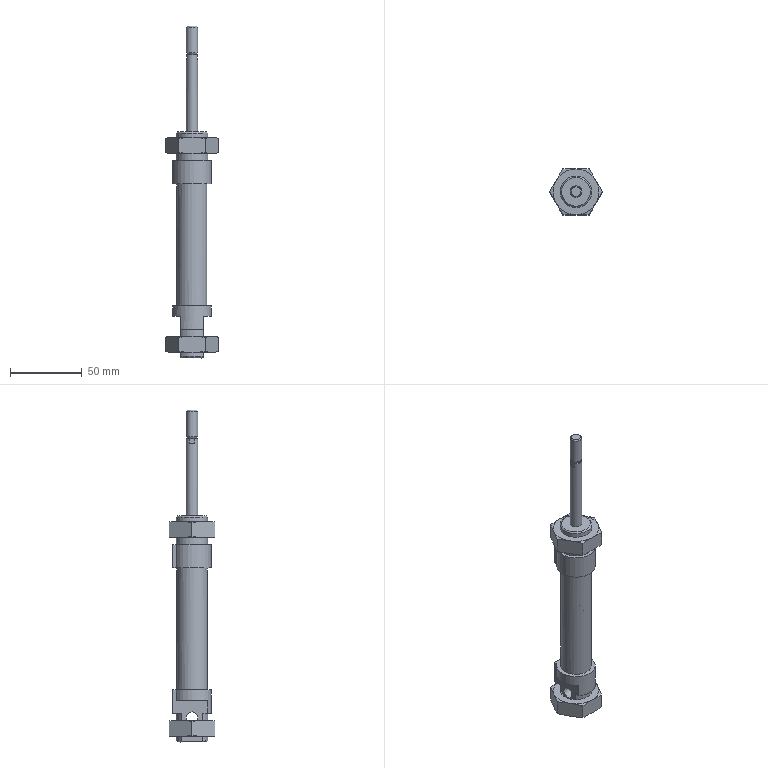Part | STEP file | 19210 DSNU-20-50-P-A-----(asm_0_1) | 4 solids | 94 faces | box 36.95 x 32 x 232 mm | volume 60932 mm3 | plane 43 | cone 35 | cylinder 16 | commonest cylinder face diameters 8 x4 22 x3 8.566 x2 20 x2 20.16 x2 27 x2